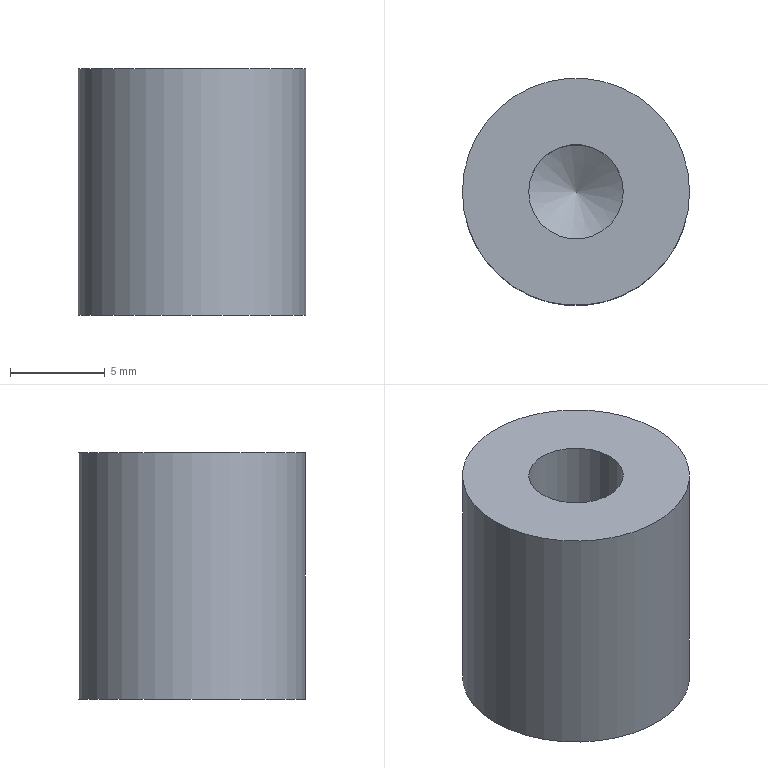Part | NX | 1 solid | 5 faces | box 12 x 12 x 13 mm | volume 1303 mm3 | cylinder 2 | plane 2 | cone 1 | commonest cylinder face diameters 5 x1 12 x1
STEP:
#1=CARTESIAN_POINT('',(-2.5,0.,5.));
#2=VERTEX_POINT('',#1);
#3=CARTESIAN_POINT('',(0.,0.,5.));
#4=DIRECTION('',(0.,0.,-1.));
#5=DIRECTION('',(-1.,0.,0.));
#6=AXIS2_PLACEMENT_3D('',#3,#4,#5);
#7=CIRCLE('',#6,2.5);
#8=EDGE_CURVE('',#2,#2,#7,.T.);
#9=ORIENTED_EDGE('',*,*,#8,.F.);
#10=EDGE_LOOP('',(#9));
#11=FACE_BOUND('',#10,.T.);
#12=CARTESIAN_POINT('',(0.,0.,3.498));
#13=VERTEX_POINT('',#12);
#14=VERTEX_LOOP('',#13);
#15=FACE_BOUND('',#14,.T.);
#16=CARTESIAN_POINT('',(0.,0.,3.498));
#17=DIRECTION('',(0.,0.,1.));
#18=DIRECTION('',(-1.,0.,0.));
#19=AXIS2_PLACEMENT_3D('',#16,#17,#18);
#20=CONICAL_SURFACE('',#19,0.,59.);
#21=ADVANCED_FACE('',(#11,#15),#20,.F.);
#22=CARTESIAN_POINT('',(-2.5,0.,13.));
#23=VERTEX_POINT('',#22);
#24=CARTESIAN_POINT('',(0.,0.,13.));
#25=DIRECTION('',(0.,0.,-1.));
#26=DIRECTION('',(-1.,0.,0.));
#27=AXIS2_PLACEMENT_3D('',#24,#25,#26);
#28=CIRCLE('',#27,2.5);
#29=EDGE_CURVE('',#23,#23,#28,.T.);
#30=ORIENTED_EDGE('',*,*,#29,.F.);
#31=EDGE_LOOP('',(#30));
#32=FACE_BOUND('',#31,.T.);
#33=ORIENTED_EDGE('',*,*,#8,.T.);
#34=EDGE_LOOP('',(#33));
#35=FACE_BOUND('',#34,.T.);
#36=CARTESIAN_POINT('',(0.,0.,13.));
#37=DIRECTION('',(0.,0.,-1.));
#38=DIRECTION('',(1.,0.,0.));
#39=AXIS2_PLACEMENT_3D('',#36,#37,#38);
#40=CYLINDRICAL_SURFACE('',#39,2.5);
#41=ADVANCED_FACE('',(#32,#35),#40,.F.);
#42=CARTESIAN_POINT('',(-6.,0.,13.));
#43=VERTEX_POINT('',#42);
#44=CARTESIAN_POINT('',(0.,0.,13.));
#45=DIRECTION('',(0.,0.,-1.));
#46=DIRECTION('',(-1.,0.,0.));
#47=AXIS2_PLACEMENT_3D('',#44,#45,#46);
#48=CIRCLE('',#47,6.);
#49=EDGE_CURVE('',#43,#43,#48,.T.);
#50=ORIENTED_EDGE('',*,*,#49,.F.);
#51=EDGE_LOOP('',(#50));
#52=FACE_BOUND('',#51,.T.);
#53=ORIENTED_EDGE('',*,*,#29,.T.);
#54=EDGE_LOOP('',(#53));
#55=FACE_BOUND('',#54,.T.);
#56=CARTESIAN_POINT('',(0.,2.5,13.));
#57=DIRECTION('',(0.,0.,-1.));
#58=DIRECTION('',(1.,0.,0.));
#59=AXIS2_PLACEMENT_3D('',#56,#57,#58);
#60=PLANE('',#59);
#61=ADVANCED_FACE('',(#52,#55),#60,.F.);
#62=CARTESIAN_POINT('',(-6.,0.,0.));
#63=VERTEX_POINT('',#62);
#64=CARTESIAN_POINT('',(0.,0.,0.));
#65=DIRECTION('',(0.,0.,-1.));
#66=DIRECTION('',(-1.,0.,0.));
#67=AXIS2_PLACEMENT_3D('',#64,#65,#66);
#68=CIRCLE('',#67,6.);
#69=EDGE_CURVE('',#63,#63,#68,.T.);
#70=ORIENTED_EDGE('',*,*,#69,.F.);
#71=EDGE_LOOP('',(#70));
#72=FACE_BOUND('',#71,.T.);
#73=ORIENTED_EDGE('',*,*,#49,.T.);
#74=EDGE_LOOP('',(#73));
#75=FACE_BOUND('',#74,.T.);
#76=CARTESIAN_POINT('',(0.,0.,13.));
#77=DIRECTION('',(0.,0.,-1.));
#78=DIRECTION('',(1.,0.,0.));
#79=AXIS2_PLACEMENT_3D('',#76,#77,#78);
#80=CYLINDRICAL_SURFACE('',#79,6.);
#81=ADVANCED_FACE('',(#72,#75),#80,.T.);
#82=ORIENTED_EDGE('',*,*,#69,.T.);
#83=EDGE_LOOP('',(#82));
#84=FACE_OUTER_BOUND('',#83,.T.);
#85=CARTESIAN_POINT('',(0.,6.,0.));
#86=DIRECTION('',(0.,0.,1.));
#87=DIRECTION('',(-1.,0.,0.));
#88=AXIS2_PLACEMENT_3D('',#85,#86,#87);
#89=PLANE('',#88);
#90=ADVANCED_FACE('',(#84),#89,.F.);
#91=CLOSED_SHELL('',(#21,#41,#61,#81,#90));
#92=MANIFOLD_SOLID_BREP('',#91);
#93=(LENGTH_UNIT()NAMED_UNIT(*)SI_UNIT(.MILLI.,.METRE.));
#94=UNCERTAINTY_MEASURE_WITH_UNIT(LENGTH_MEASURE(0.00002),#93,'','');
#95=(NAMED_UNIT(*)PLANE_ANGLE_UNIT()SI_UNIT($,.RADIAN.));
#96=PLANE_ANGLE_MEASURE_WITH_UNIT(PLANE_ANGLE_MEASURE(0.01745),#95);
#97=DIMENSIONAL_EXPONENTS(0.,0.,0.,0.,0.,0.,0.);
#98=(CONVERSION_BASED_UNIT('DEGREE',#96)NAMED_UNIT(#97)PLANE_ANGLE_UNIT());
#99=(NAMED_UNIT(*)SI_UNIT($,.STERADIAN.)SOLID_ANGLE_UNIT());
#100=(GEOMETRIC_REPRESENTATION_CONTEXT(3)GLOBAL_UNCERTAINTY_ASSIGNED_CONTEXT((#94))GLOBAL_UNIT_ASSIGNED_CONTEXT((#93,#98,#99))REPRESENTATION_CONTEXT('',''));
#101=ADVANCED_BREP_SHAPE_REPRESENTATION('',(#92),#100);